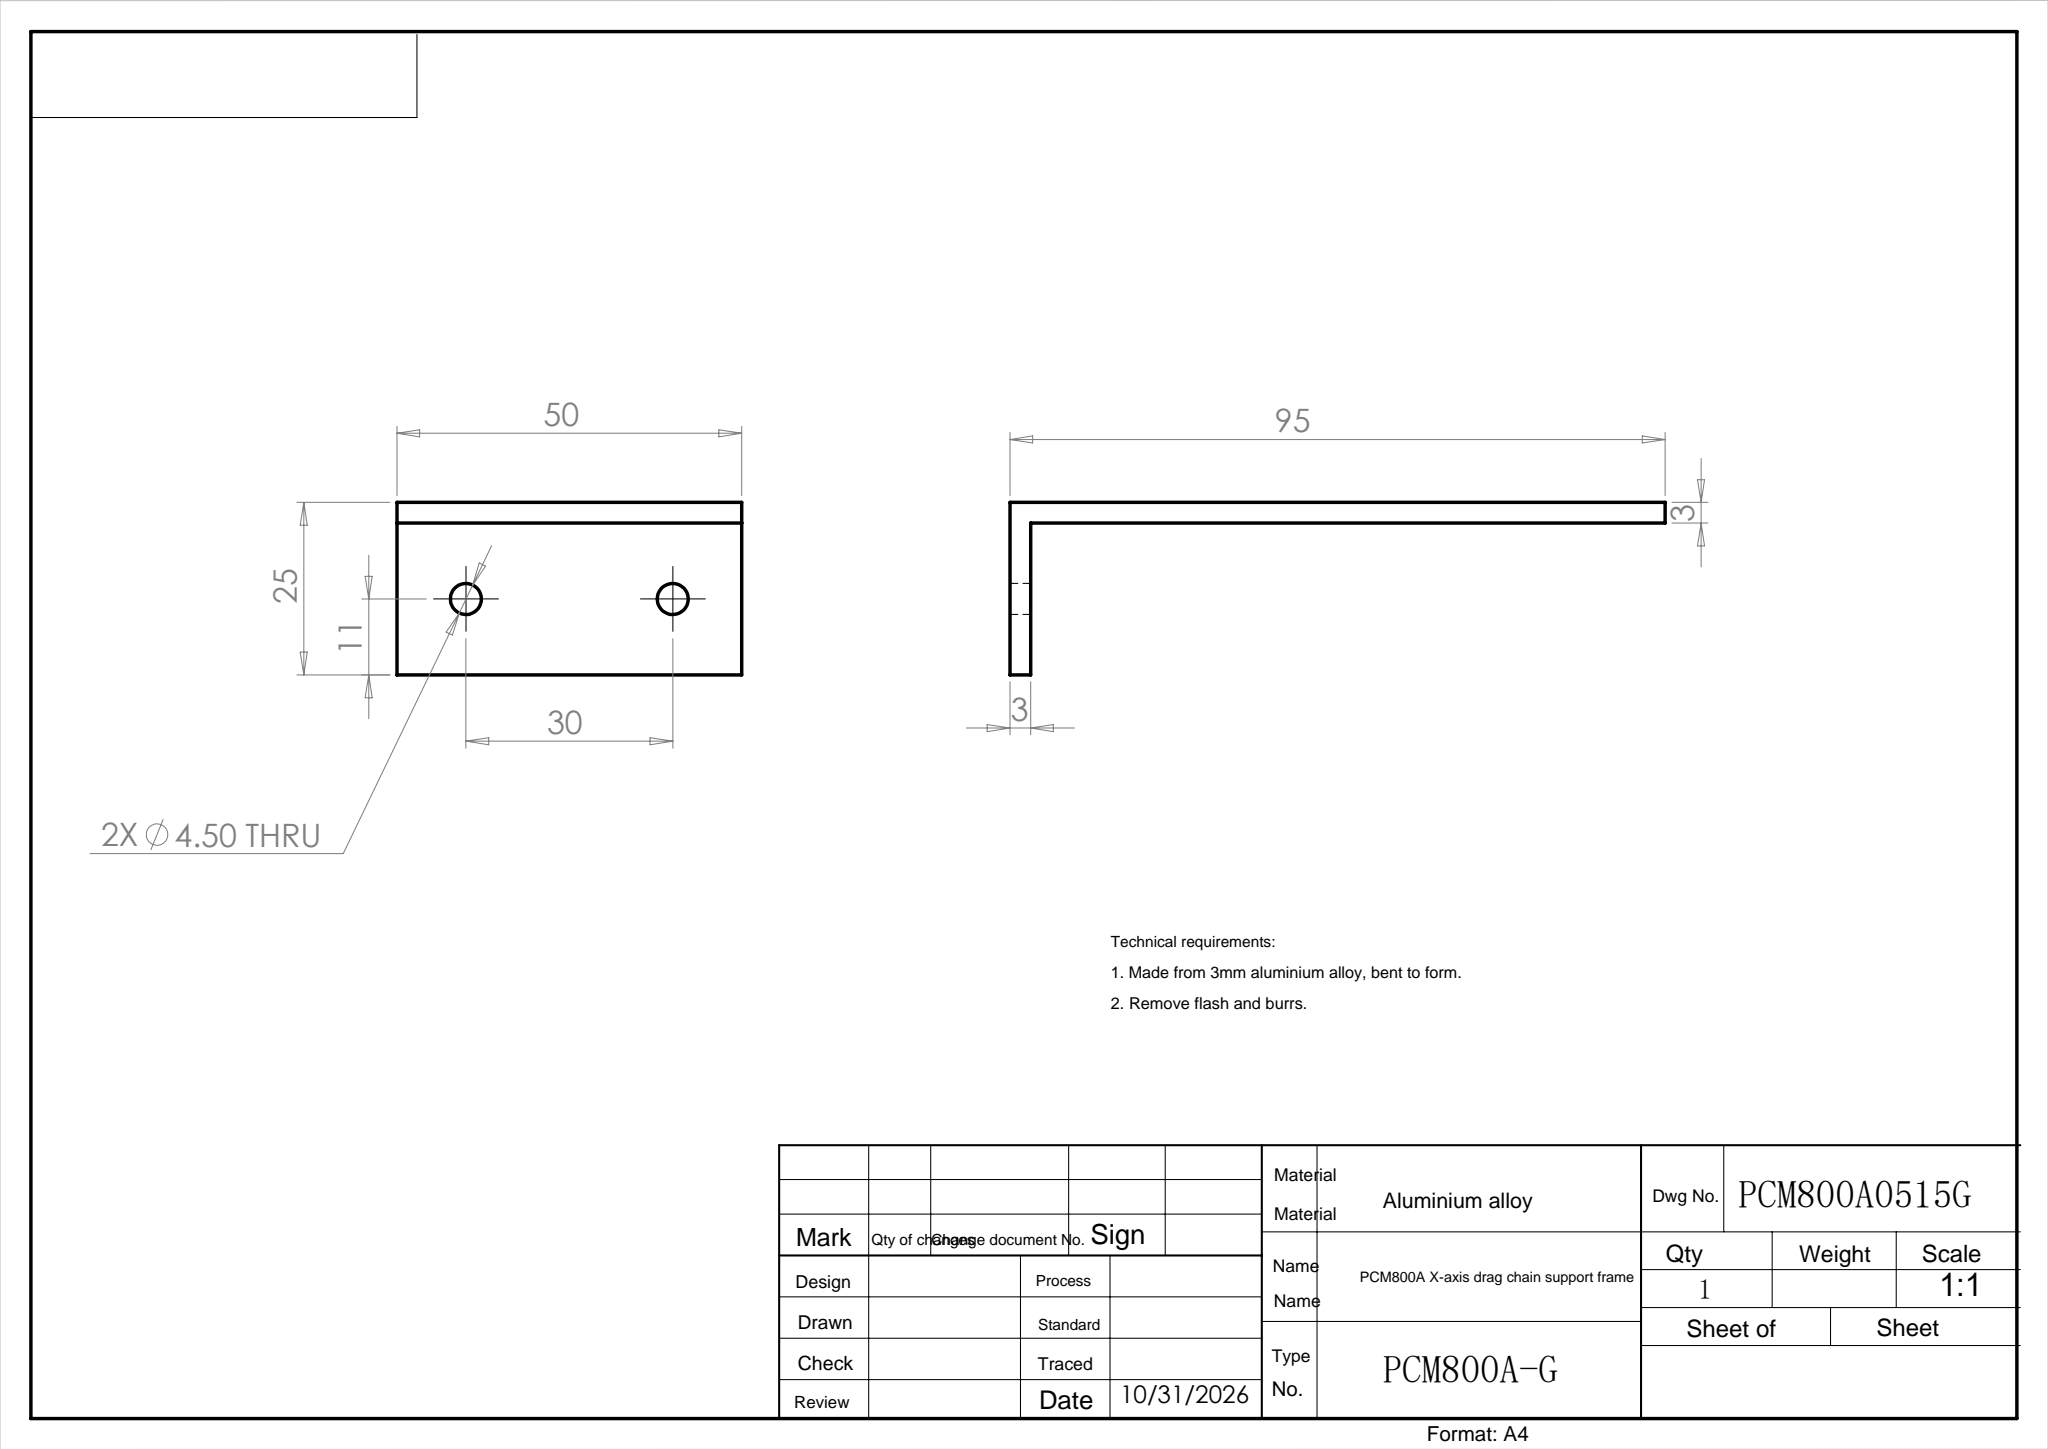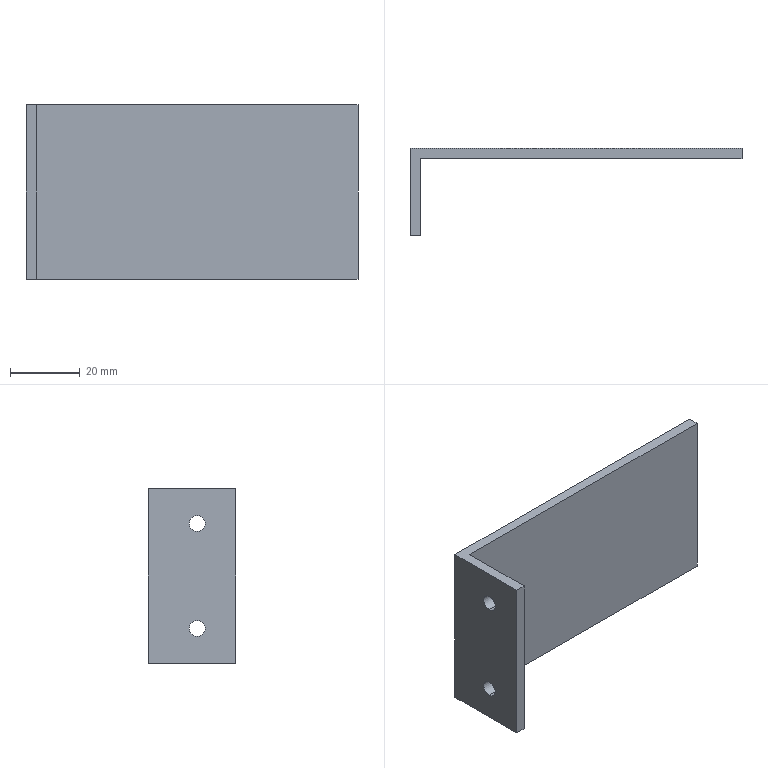Part | SolidWorks | features ExtruThin 1, ICE 1 | 1 solid | 12 faces | box 95 x 25 x 50 mm | volume 17455 mm3 | plane 8 | cylinder 4 | commonest cylinder face diameters 4.5 x4
STEP:
#1=CARTESIAN_POINT('',(0.,11.,7.75));
#2=VERTEX_POINT('',#1);
#3=CARTESIAN_POINT('',(0.,11.,12.25));
#4=VERTEX_POINT('',#3);
#5=CARTESIAN_POINT('',(0.,11.,10.));
#6=DIRECTION('',(-1.,0.,0.));
#7=DIRECTION('',(0.,0.,1.));
#8=AXIS2_PLACEMENT_3D('',#5,#6,#7);
#9=CIRCLE('',#8,2.25);
#10=EDGE_CURVE('',#2,#4,#9,.T.);
#11=ORIENTED_EDGE('',*,*,#10,.T.);
#12=CARTESIAN_POINT('',(3.,11.,12.25));
#13=VERTEX_POINT('',#12);
#14=CARTESIAN_POINT('',(-7.,11.,12.25));
#15=DIRECTION('',(1.,0.,0.));
#16=VECTOR('',#15,1000.);
#17=LINE('',#14,#16);
#18=EDGE_CURVE('',#4,#13,#17,.T.);
#19=ORIENTED_EDGE('',*,*,#18,.T.);
#20=CARTESIAN_POINT('',(3.,11.,7.75));
#21=VERTEX_POINT('',#20);
#22=CARTESIAN_POINT('',(3.,11.,10.));
#23=DIRECTION('',(1.,0.,0.));
#24=DIRECTION('',(0.,0.,1.));
#25=AXIS2_PLACEMENT_3D('',#22,#23,#24);
#26=CIRCLE('',#25,2.25);
#27=EDGE_CURVE('',#13,#21,#26,.T.);
#28=ORIENTED_EDGE('',*,*,#27,.T.);
#29=CARTESIAN_POINT('',(-7.,11.,7.75));
#30=DIRECTION('',(1.,0.,0.));
#31=VECTOR('',#30,1000.);
#32=LINE('',#29,#31);
#33=EDGE_CURVE('',#2,#21,#32,.T.);
#34=ORIENTED_EDGE('',*,*,#33,.F.);
#35=EDGE_LOOP('',(#11,#19,#28,#34));
#36=FACE_OUTER_BOUND('',#35,.T.);
#37=CARTESIAN_POINT('',(-7.,11.,10.));
#38=DIRECTION('',(1.,0.,0.));
#39=DIRECTION('',(0.,0.,-1.));
#40=AXIS2_PLACEMENT_3D('',#37,#38,#39);
#41=CYLINDRICAL_SURFACE('',#40,2.25);
#42=ADVANCED_FACE('',(#36),#41,.F.);
#43=CARTESIAN_POINT('',(0.,11.,37.75));
#44=VERTEX_POINT('',#43);
#45=CARTESIAN_POINT('',(0.,11.,42.25));
#46=VERTEX_POINT('',#45);
#47=CARTESIAN_POINT('',(0.,11.,40.));
#48=DIRECTION('',(-1.,0.,0.));
#49=DIRECTION('',(0.,0.,1.));
#50=AXIS2_PLACEMENT_3D('',#47,#48,#49);
#51=CIRCLE('',#50,2.25);
#52=EDGE_CURVE('',#44,#46,#51,.T.);
#53=ORIENTED_EDGE('',*,*,#52,.T.);
#54=CARTESIAN_POINT('',(3.,11.,42.25));
#55=VERTEX_POINT('',#54);
#56=CARTESIAN_POINT('',(-7.,11.,42.25));
#57=DIRECTION('',(1.,0.,0.));
#58=VECTOR('',#57,1000.);
#59=LINE('',#56,#58);
#60=EDGE_CURVE('',#46,#55,#59,.T.);
#61=ORIENTED_EDGE('',*,*,#60,.T.);
#62=CARTESIAN_POINT('',(3.,11.,37.75));
#63=VERTEX_POINT('',#62);
#64=CARTESIAN_POINT('',(3.,11.,40.));
#65=DIRECTION('',(1.,0.,0.));
#66=DIRECTION('',(0.,0.,-1.));
#67=AXIS2_PLACEMENT_3D('',#64,#65,#66);
#68=CIRCLE('',#67,2.25);
#69=EDGE_CURVE('',#55,#63,#68,.T.);
#70=ORIENTED_EDGE('',*,*,#69,.T.);
#71=CARTESIAN_POINT('',(-7.,11.,37.75));
#72=DIRECTION('',(1.,0.,0.));
#73=VECTOR('',#72,1000.);
#74=LINE('',#71,#73);
#75=EDGE_CURVE('',#44,#63,#74,.T.);
#76=ORIENTED_EDGE('',*,*,#75,.F.);
#77=EDGE_LOOP('',(#53,#61,#70,#76));
#78=FACE_OUTER_BOUND('',#77,.T.);
#79=CARTESIAN_POINT('',(-7.,11.,40.));
#80=DIRECTION('',(1.,0.,0.));
#81=DIRECTION('',(0.,0.,-1.));
#82=AXIS2_PLACEMENT_3D('',#79,#80,#81);
#83=CYLINDRICAL_SURFACE('',#82,2.25);
#84=ADVANCED_FACE('',(#78),#83,.F.);
#85=CARTESIAN_POINT('',(3.,22.,0.));
#86=VERTEX_POINT('',#85);
#87=CARTESIAN_POINT('',(95.,22.,0.));
#88=VERTEX_POINT('',#87);
#89=CARTESIAN_POINT('',(0.,22.,0.));
#90=DIRECTION('',(1.,0.,0.));
#91=VECTOR('',#90,1000.);
#92=LINE('',#89,#91);
#93=EDGE_CURVE('',#86,#88,#92,.T.);
#94=ORIENTED_EDGE('',*,*,#93,.T.);
#95=CARTESIAN_POINT('',(95.,22.,50.));
#96=VERTEX_POINT('',#95);
#97=CARTESIAN_POINT('',(95.,22.,50.));
#98=DIRECTION('',(0.,0.,-1.));
#99=VECTOR('',#98,1000.);
#100=LINE('',#97,#99);
#101=EDGE_CURVE('',#96,#88,#100,.T.);
#102=ORIENTED_EDGE('',*,*,#101,.F.);
#103=CARTESIAN_POINT('',(3.,22.,50.));
#104=VERTEX_POINT('',#103);
#105=CARTESIAN_POINT('',(0.,22.,50.));
#106=DIRECTION('',(1.,0.,0.));
#107=VECTOR('',#106,1000.);
#108=LINE('',#105,#107);
#109=EDGE_CURVE('',#104,#96,#108,.T.);
#110=ORIENTED_EDGE('',*,*,#109,.F.);
#111=CARTESIAN_POINT('',(3.,22.,50.));
#112=DIRECTION('',(0.,0.,-1.));
#113=VECTOR('',#112,1000.);
#114=LINE('',#111,#113);
#115=EDGE_CURVE('',#104,#86,#114,.T.);
#116=ORIENTED_EDGE('',*,*,#115,.T.);
#117=EDGE_LOOP('',(#94,#102,#110,#116));
#118=FACE_OUTER_BOUND('',#117,.T.);
#119=CARTESIAN_POINT('',(0.,22.,50.));
#120=DIRECTION('',(0.,1.,0.));
#121=DIRECTION('',(0.,0.,1.));
#122=AXIS2_PLACEMENT_3D('',#119,#120,#121);
#123=PLANE('',#122);
#124=ADVANCED_FACE('',(#118),#123,.F.);
#125=CARTESIAN_POINT('',(95.,25.,0.));
#126=VERTEX_POINT('',#125);
#127=CARTESIAN_POINT('',(95.,25.,0.));
#128=DIRECTION('',(0.,-1.,0.));
#129=VECTOR('',#128,1000.);
#130=LINE('',#127,#129);
#131=EDGE_CURVE('',#126,#88,#130,.T.);
#132=ORIENTED_EDGE('',*,*,#131,.F.);
#133=CARTESIAN_POINT('',(95.,25.,50.));
#134=VERTEX_POINT('',#133);
#135=CARTESIAN_POINT('',(95.,25.,50.));
#136=DIRECTION('',(0.,0.,-1.));
#137=VECTOR('',#136,1000.);
#138=LINE('',#135,#137);
#139=EDGE_CURVE('',#134,#126,#138,.T.);
#140=ORIENTED_EDGE('',*,*,#139,.F.);
#141=CARTESIAN_POINT('',(95.,25.,50.));
#142=DIRECTION('',(0.,-1.,0.));
#143=VECTOR('',#142,1000.);
#144=LINE('',#141,#143);
#145=EDGE_CURVE('',#134,#96,#144,.T.);
#146=ORIENTED_EDGE('',*,*,#145,.T.);
#147=ORIENTED_EDGE('',*,*,#101,.T.);
#148=EDGE_LOOP('',(#132,#140,#146,#147));
#149=FACE_OUTER_BOUND('',#148,.T.);
#150=CARTESIAN_POINT('',(95.,25.,50.));
#151=DIRECTION('',(1.,0.,0.));
#152=DIRECTION('',(0.,0.,-1.));
#153=AXIS2_PLACEMENT_3D('',#150,#151,#152);
#154=PLANE('',#153);
#155=ADVANCED_FACE('',(#149),#154,.T.);
#156=CARTESIAN_POINT('',(0.,25.,0.));
#157=VERTEX_POINT('',#156);
#158=CARTESIAN_POINT('',(0.,25.,0.));
#159=DIRECTION('',(1.,0.,0.));
#160=VECTOR('',#159,1000.);
#161=LINE('',#158,#160);
#162=EDGE_CURVE('',#157,#126,#161,.T.);
#163=ORIENTED_EDGE('',*,*,#162,.F.);
#164=CARTESIAN_POINT('',(0.,25.,50.));
#165=VERTEX_POINT('',#164);
#166=CARTESIAN_POINT('',(0.,25.,50.));
#167=DIRECTION('',(0.,0.,-1.));
#168=VECTOR('',#167,1000.);
#169=LINE('',#166,#168);
#170=EDGE_CURVE('',#165,#157,#169,.T.);
#171=ORIENTED_EDGE('',*,*,#170,.F.);
#172=CARTESIAN_POINT('',(0.,25.,50.));
#173=DIRECTION('',(1.,0.,0.));
#174=VECTOR('',#173,1000.);
#175=LINE('',#172,#174);
#176=EDGE_CURVE('',#165,#134,#175,.T.);
#177=ORIENTED_EDGE('',*,*,#176,.T.);
#178=ORIENTED_EDGE('',*,*,#139,.T.);
#179=EDGE_LOOP('',(#163,#171,#177,#178));
#180=FACE_OUTER_BOUND('',#179,.T.);
#181=CARTESIAN_POINT('',(0.,25.,50.));
#182=DIRECTION('',(0.,1.,0.));
#183=DIRECTION('',(0.,0.,1.));
#184=AXIS2_PLACEMENT_3D('',#181,#182,#183);
#185=PLANE('',#184);
#186=ADVANCED_FACE('',(#180),#185,.T.);
#187=ORIENTED_EDGE('',*,*,#10,.F.);
#188=CARTESIAN_POINT('',(0.,11.,10.));
#189=DIRECTION('',(-1.,0.,0.));
#190=DIRECTION('',(0.,0.,1.));
#191=AXIS2_PLACEMENT_3D('',#188,#189,#190);
#192=CIRCLE('',#191,2.25);
#193=EDGE_CURVE('',#4,#2,#192,.T.);
#194=ORIENTED_EDGE('',*,*,#193,.F.);
#195=EDGE_LOOP('',(#187,#194));
#196=FACE_BOUND('',#195,.T.);
#197=ORIENTED_EDGE('',*,*,#52,.F.);
#198=CARTESIAN_POINT('',(0.,11.,40.));
#199=DIRECTION('',(-1.,0.,0.));
#200=DIRECTION('',(0.,0.,1.));
#201=AXIS2_PLACEMENT_3D('',#198,#199,#200);
#202=CIRCLE('',#201,2.25);
#203=EDGE_CURVE('',#46,#44,#202,.T.);
#204=ORIENTED_EDGE('',*,*,#203,.F.);
#205=EDGE_LOOP('',(#197,#204));
#206=FACE_BOUND('',#205,.T.);
#207=CARTESIAN_POINT('',(0.,0.,0.));
#208=VERTEX_POINT('',#207);
#209=CARTESIAN_POINT('',(0.,0.,0.));
#210=DIRECTION('',(0.,1.,0.));
#211=VECTOR('',#210,1000.);
#212=LINE('',#209,#211);
#213=EDGE_CURVE('',#208,#157,#212,.T.);
#214=ORIENTED_EDGE('',*,*,#213,.F.);
#215=CARTESIAN_POINT('',(0.,0.,50.));
#216=VERTEX_POINT('',#215);
#217=CARTESIAN_POINT('',(0.,0.,50.));
#218=DIRECTION('',(0.,0.,-1.));
#219=VECTOR('',#218,1000.);
#220=LINE('',#217,#219);
#221=EDGE_CURVE('',#216,#208,#220,.T.);
#222=ORIENTED_EDGE('',*,*,#221,.F.);
#223=CARTESIAN_POINT('',(0.,0.,50.));
#224=DIRECTION('',(0.,1.,0.));
#225=VECTOR('',#224,1000.);
#226=LINE('',#223,#225);
#227=EDGE_CURVE('',#216,#165,#226,.T.);
#228=ORIENTED_EDGE('',*,*,#227,.T.);
#229=ORIENTED_EDGE('',*,*,#170,.T.);
#230=EDGE_LOOP('',(#214,#222,#228,#229));
#231=FACE_OUTER_BOUND('',#230,.T.);
#232=CARTESIAN_POINT('',(0.,0.,50.));
#233=DIRECTION('',(-1.,0.,0.));
#234=DIRECTION('',(0.,0.,1.));
#235=AXIS2_PLACEMENT_3D('',#232,#233,#234);
#236=PLANE('',#235);
#237=ADVANCED_FACE('',(#196,#206,#231),#236,.T.);
#238=CARTESIAN_POINT('',(3.,0.,0.));
#239=VERTEX_POINT('',#238);
#240=CARTESIAN_POINT('',(3.,0.,0.));
#241=DIRECTION('',(-1.,0.,0.));
#242=VECTOR('',#241,1000.);
#243=LINE('',#240,#242);
#244=EDGE_CURVE('',#239,#208,#243,.T.);
#245=ORIENTED_EDGE('',*,*,#244,.F.);
#246=CARTESIAN_POINT('',(3.,0.,50.));
#247=VERTEX_POINT('',#246);
#248=CARTESIAN_POINT('',(3.,0.,50.));
#249=DIRECTION('',(0.,0.,-1.));
#250=VECTOR('',#249,1000.);
#251=LINE('',#248,#250);
#252=EDGE_CURVE('',#247,#239,#251,.T.);
#253=ORIENTED_EDGE('',*,*,#252,.F.);
#254=CARTESIAN_POINT('',(3.,0.,50.));
#255=DIRECTION('',(-1.,0.,0.));
#256=VECTOR('',#255,1000.);
#257=LINE('',#254,#256);
#258=EDGE_CURVE('',#247,#216,#257,.T.);
#259=ORIENTED_EDGE('',*,*,#258,.T.);
#260=ORIENTED_EDGE('',*,*,#221,.T.);
#261=EDGE_LOOP('',(#245,#253,#259,#260));
#262=FACE_OUTER_BOUND('',#261,.T.);
#263=CARTESIAN_POINT('',(3.,0.,50.));
#264=DIRECTION('',(0.,-1.,0.));
#265=DIRECTION('',(0.,0.,-1.));
#266=AXIS2_PLACEMENT_3D('',#263,#264,#265);
#267=PLANE('',#266);
#268=ADVANCED_FACE('',(#262),#267,.T.);
#269=CARTESIAN_POINT('',(3.,11.,10.));
#270=DIRECTION('',(1.,0.,0.));
#271=DIRECTION('',(0.,0.,1.));
#272=AXIS2_PLACEMENT_3D('',#269,#270,#271);
#273=CIRCLE('',#272,2.25);
#274=EDGE_CURVE('',#21,#13,#273,.T.);
#275=ORIENTED_EDGE('',*,*,#274,.F.);
#276=ORIENTED_EDGE('',*,*,#27,.F.);
#277=EDGE_LOOP('',(#275,#276));
#278=FACE_BOUND('',#277,.T.);
#279=CARTESIAN_POINT('',(3.,11.,40.));
#280=DIRECTION('',(1.,0.,0.));
#281=DIRECTION('',(0.,0.,-1.));
#282=AXIS2_PLACEMENT_3D('',#279,#280,#281);
#283=CIRCLE('',#282,2.25);
#284=EDGE_CURVE('',#63,#55,#283,.T.);
#285=ORIENTED_EDGE('',*,*,#284,.F.);
#286=ORIENTED_EDGE('',*,*,#69,.F.);
#287=EDGE_LOOP('',(#285,#286));
#288=FACE_BOUND('',#287,.T.);
#289=CARTESIAN_POINT('',(3.,0.,0.));
#290=DIRECTION('',(0.,1.,0.));
#291=VECTOR('',#290,1000.);
#292=LINE('',#289,#291);
#293=EDGE_CURVE('',#239,#86,#292,.T.);
#294=ORIENTED_EDGE('',*,*,#293,.T.);
#295=ORIENTED_EDGE('',*,*,#115,.F.);
#296=CARTESIAN_POINT('',(3.,0.,50.));
#297=DIRECTION('',(0.,1.,0.));
#298=VECTOR('',#297,1000.);
#299=LINE('',#296,#298);
#300=EDGE_CURVE('',#247,#104,#299,.T.);
#301=ORIENTED_EDGE('',*,*,#300,.F.);
#302=ORIENTED_EDGE('',*,*,#252,.T.);
#303=EDGE_LOOP('',(#294,#295,#301,#302));
#304=FACE_OUTER_BOUND('',#303,.T.);
#305=CARTESIAN_POINT('',(3.,0.,50.));
#306=DIRECTION('',(-1.,0.,0.));
#307=DIRECTION('',(0.,0.,1.));
#308=AXIS2_PLACEMENT_3D('',#305,#306,#307);
#309=PLANE('',#308);
#310=ADVANCED_FACE('',(#278,#288,#304),#309,.F.);
#311=ORIENTED_EDGE('',*,*,#109,.T.);
#312=ORIENTED_EDGE('',*,*,#145,.F.);
#313=ORIENTED_EDGE('',*,*,#176,.F.);
#314=ORIENTED_EDGE('',*,*,#227,.F.);
#315=ORIENTED_EDGE('',*,*,#258,.F.);
#316=ORIENTED_EDGE('',*,*,#300,.T.);
#317=EDGE_LOOP('',(#311,#312,#313,#314,#315,#316));
#318=FACE_OUTER_BOUND('',#317,.T.);
#319=CARTESIAN_POINT('',(95.,22.,50.));
#320=DIRECTION('',(0.,0.,-1.));
#321=DIRECTION('',(-1.,0.,0.));
#322=AXIS2_PLACEMENT_3D('',#319,#320,#321);
#323=PLANE('',#322);
#324=ADVANCED_FACE('',(#318),#323,.F.);
#325=ORIENTED_EDGE('',*,*,#93,.F.);
#326=ORIENTED_EDGE('',*,*,#293,.F.);
#327=ORIENTED_EDGE('',*,*,#244,.T.);
#328=ORIENTED_EDGE('',*,*,#213,.T.);
#329=ORIENTED_EDGE('',*,*,#162,.T.);
#330=ORIENTED_EDGE('',*,*,#131,.T.);
#331=EDGE_LOOP('',(#325,#326,#327,#328,#329,#330));
#332=FACE_OUTER_BOUND('',#331,.T.);
#333=CARTESIAN_POINT('',(95.,22.,0.));
#334=DIRECTION('',(0.,0.,-1.));
#335=DIRECTION('',(-1.,0.,0.));
#336=AXIS2_PLACEMENT_3D('',#333,#334,#335);
#337=PLANE('',#336);
#338=ADVANCED_FACE('',(#332),#337,.T.);
#339=ORIENTED_EDGE('',*,*,#60,.F.);
#340=ORIENTED_EDGE('',*,*,#203,.T.);
#341=ORIENTED_EDGE('',*,*,#75,.T.);
#342=ORIENTED_EDGE('',*,*,#284,.T.);
#343=EDGE_LOOP('',(#339,#340,#341,#342));
#344=FACE_OUTER_BOUND('',#343,.T.);
#345=CARTESIAN_POINT('',(-7.,11.,40.));
#346=DIRECTION('',(1.,0.,0.));
#347=DIRECTION('',(0.,0.,-1.));
#348=AXIS2_PLACEMENT_3D('',#345,#346,#347);
#349=CYLINDRICAL_SURFACE('',#348,2.25);
#350=ADVANCED_FACE('',(#344),#349,.F.);
#351=ORIENTED_EDGE('',*,*,#18,.F.);
#352=ORIENTED_EDGE('',*,*,#193,.T.);
#353=ORIENTED_EDGE('',*,*,#33,.T.);
#354=ORIENTED_EDGE('',*,*,#274,.T.);
#355=EDGE_LOOP('',(#351,#352,#353,#354));
#356=FACE_OUTER_BOUND('',#355,.T.);
#357=CARTESIAN_POINT('',(-7.,11.,10.));
#358=DIRECTION('',(1.,0.,0.));
#359=DIRECTION('',(0.,0.,-1.));
#360=AXIS2_PLACEMENT_3D('',#357,#358,#359);
#361=CYLINDRICAL_SURFACE('',#360,2.25);
#362=ADVANCED_FACE('',(#356),#361,.F.);
#363=CLOSED_SHELL('',(#42,#84,#124,#155,#186,#237,#268,#310,#324,#338,#350,#362));
#364=MANIFOLD_SOLID_BREP('',#363);
#365=CARTESIAN_POINT('',(0.,0.,0.));
#366=DIRECTION('',(0.,0.,1.));
#367=DIRECTION('',(1.,0.,0.));
#368=AXIS2_PLACEMENT_3D('',#365,#366,#367);
#369=(LENGTH_UNIT()NAMED_UNIT(*)SI_UNIT(.MILLI.,.METRE.));
#370=UNCERTAINTY_MEASURE_WITH_UNIT(LENGTH_MEASURE(0.00001),#369,'','');
#371=(NAMED_UNIT(*)PLANE_ANGLE_UNIT()SI_UNIT($,.RADIAN.));
#372=(NAMED_UNIT(*)SI_UNIT($,.STERADIAN.)SOLID_ANGLE_UNIT());
#373=(GEOMETRIC_REPRESENTATION_CONTEXT(3)GLOBAL_UNCERTAINTY_ASSIGNED_CONTEXT((#370))GLOBAL_UNIT_ASSIGNED_CONTEXT((#369,#371,#372))REPRESENTATION_CONTEXT('',''));
#374=ADVANCED_BREP_SHAPE_REPRESENTATION('',(#364,#368),#373);